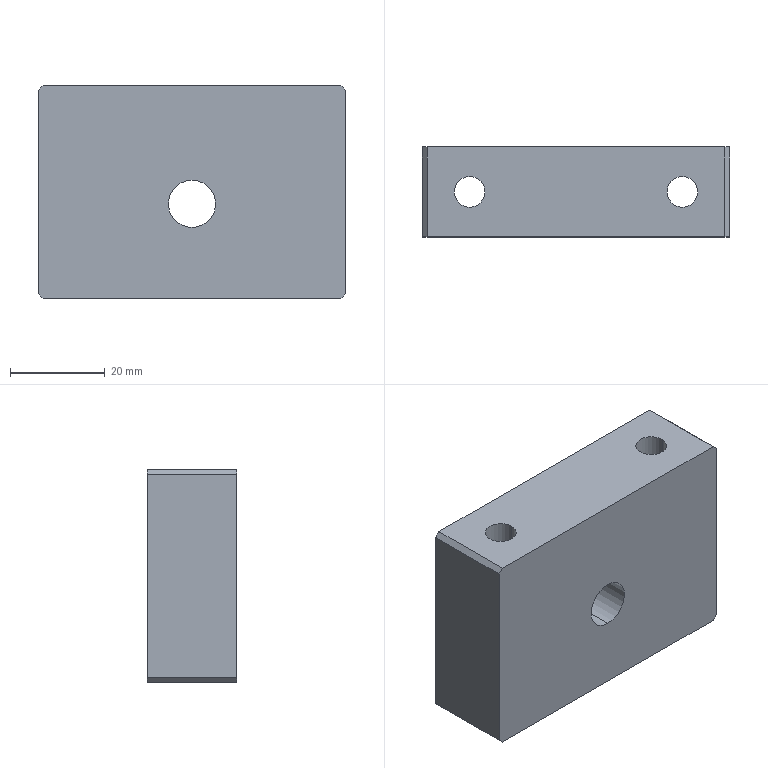Part | STEP file | Guide rod fixing plate 2 | 1 solid | 29 faces | box 65 x 19 x 45 mm | volume 44231 mm3 | cylinder 14 | plane 13 | cone 2 | commonest cylinder face diameters 6.5 x4 12 x4 4.2 x2 10 x2 20 x2